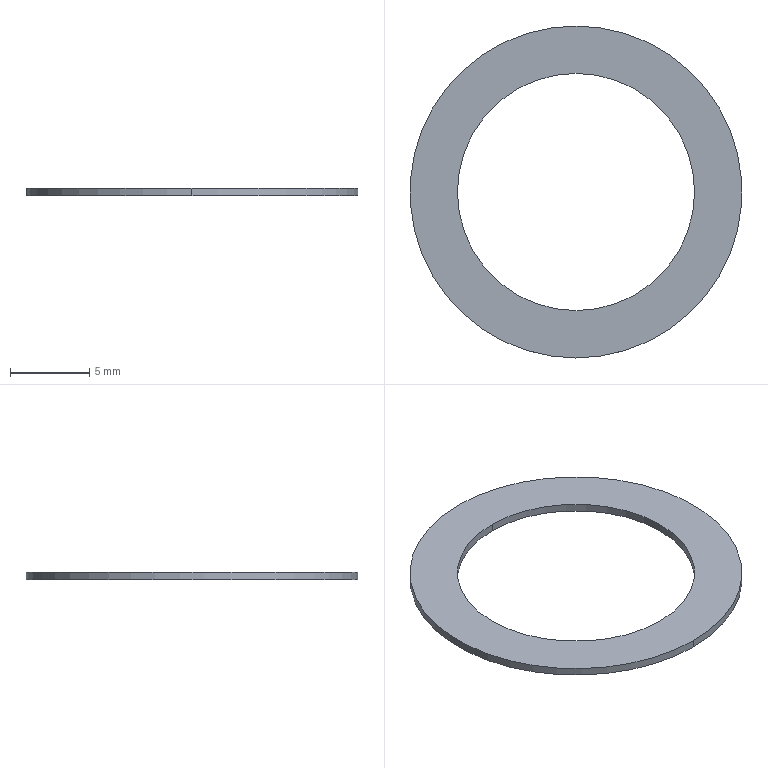Part | STEP file | MSBR-19_1_1_1_1 | 1 solid | 6 faces | box 21 x 21 x 0.5 mm | volume 84.823 mm3 | cylinder 4 | plane 2 | commonest cylinder face diameters 15 x2 21 x2
STEP:
#1=CARTESIAN_POINT('',(0.,0.,0.));
#2=DIRECTION('',(0.,0.,1.));
#3=DIRECTION('',(1.,0.,0.));
#4=AXIS2_PLACEMENT_3D('',#1,#2,#3);
#5=CARTESIAN_POINT('',(-0.000000006,7.5,22.3));
#6=VERTEX_POINT('',#5);
#7=CARTESIAN_POINT('',(-0.000000006,7.5,21.8));
#8=VERTEX_POINT('',#7);
#9=CARTESIAN_POINT('',(-0.000000006,7.5,22.3));
#10=DIRECTION('',(0.,0.,-1.));
#11=VECTOR('',#10,0.5);
#12=LINE('',#9,#11);
#13=EDGE_CURVE('',#6,#8,#12,.T.);
#14=ORIENTED_EDGE('',*,*,#13,.F.);
#15=CARTESIAN_POINT('',(-0.000000006,-7.5,22.3));
#16=VERTEX_POINT('',#15);
#17=CARTESIAN_POINT('',(-0.000000006,-0.000000021,22.3));
#18=DIRECTION('',(0.,0.,1.));
#19=DIRECTION('',(0.,-1.,0.));
#20=AXIS2_PLACEMENT_3D('',#17,#18,#19);
#21=CIRCLE('',#20,7.5);
#22=EDGE_CURVE('',#16,#6,#21,.T.);
#23=ORIENTED_EDGE('',*,*,#22,.F.);
#24=CARTESIAN_POINT('',(-0.000000006,-7.5,21.8));
#25=VERTEX_POINT('',#24);
#26=CARTESIAN_POINT('',(-0.000000006,-7.5,21.8));
#27=DIRECTION('',(0.,0.,1.));
#28=VECTOR('',#27,0.5);
#29=LINE('',#26,#28);
#30=EDGE_CURVE('',#25,#16,#29,.T.);
#31=ORIENTED_EDGE('',*,*,#30,.F.);
#32=CARTESIAN_POINT('',(-0.000000006,-0.000000021,21.8));
#33=DIRECTION('',(0.,0.,-1.));
#34=DIRECTION('',(0.,1.,0.));
#35=AXIS2_PLACEMENT_3D('',#32,#33,#34);
#36=CIRCLE('',#35,7.5);
#37=EDGE_CURVE('',#8,#25,#36,.T.);
#38=ORIENTED_EDGE('',*,*,#37,.F.);
#39=EDGE_LOOP('',(#14,#23,#31,#38));
#40=FACE_OUTER_BOUND('',#39,.F.);
#41=CARTESIAN_POINT('',(-0.000000006,-0.000000021,21.764));
#42=DIRECTION('',(0.,0.,1.));
#43=DIRECTION('',(0.,-1.,0.));
#44=AXIS2_PLACEMENT_3D('',#41,#42,#43);
#45=CYLINDRICAL_SURFACE('',#44,7.5);
#46=ADVANCED_FACE('',(#40),#45,.F.);
#47=CARTESIAN_POINT('',(-0.000000006,-0.000000021,22.3));
#48=DIRECTION('',(0.,0.,1.));
#49=DIRECTION('',(0.,1.,0.));
#50=AXIS2_PLACEMENT_3D('',#47,#48,#49);
#51=CIRCLE('',#50,7.5);
#52=EDGE_CURVE('',#6,#16,#51,.T.);
#53=ORIENTED_EDGE('',*,*,#52,.F.);
#54=ORIENTED_EDGE('',*,*,#13,.T.);
#55=CARTESIAN_POINT('',(-0.000000006,-0.000000021,21.8));
#56=DIRECTION('',(0.,0.,-1.));
#57=DIRECTION('',(0.,-1.,0.));
#58=AXIS2_PLACEMENT_3D('',#55,#56,#57);
#59=CIRCLE('',#58,7.5);
#60=EDGE_CURVE('',#25,#8,#59,.T.);
#61=ORIENTED_EDGE('',*,*,#60,.F.);
#62=ORIENTED_EDGE('',*,*,#30,.T.);
#63=EDGE_LOOP('',(#53,#54,#61,#62));
#64=FACE_OUTER_BOUND('',#63,.F.);
#65=CARTESIAN_POINT('',(-0.000000006,-0.000000021,21.764));
#66=DIRECTION('',(0.,0.,1.));
#67=DIRECTION('',(0.,1.,0.));
#68=AXIS2_PLACEMENT_3D('',#65,#66,#67);
#69=CYLINDRICAL_SURFACE('',#68,7.5);
#70=ADVANCED_FACE('',(#64),#69,.F.);
#71=CARTESIAN_POINT('',(-0.000000006,-10.5,22.3));
#72=VERTEX_POINT('',#71);
#73=CARTESIAN_POINT('',(-0.000000006,10.5,22.3));
#74=VERTEX_POINT('',#73);
#75=CARTESIAN_POINT('',(-0.000000006,-0.000000021,22.3));
#76=DIRECTION('',(0.,0.,-1.));
#77=DIRECTION('',(0.,-1.,0.));
#78=AXIS2_PLACEMENT_3D('',#75,#76,#77);
#79=CIRCLE('',#78,10.5);
#80=EDGE_CURVE('',#72,#74,#79,.T.);
#81=ORIENTED_EDGE('',*,*,#80,.T.);
#82=CARTESIAN_POINT('',(-0.000000006,-0.000000021,22.3));
#83=DIRECTION('',(0.,0.,-1.));
#84=DIRECTION('',(0.,1.,0.));
#85=AXIS2_PLACEMENT_3D('',#82,#83,#84);
#86=CIRCLE('',#85,10.5);
#87=EDGE_CURVE('',#74,#72,#86,.T.);
#88=ORIENTED_EDGE('',*,*,#87,.T.);
#89=EDGE_LOOP('',(#81,#88));
#90=FACE_OUTER_BOUND('',#89,.F.);
#91=ORIENTED_EDGE('',*,*,#22,.T.);
#92=ORIENTED_EDGE('',*,*,#52,.T.);
#93=EDGE_LOOP('',(#91,#92));
#94=FACE_BOUND('',#93,.F.);
#95=CARTESIAN_POINT('',(-0.000000006,-0.000000021,22.3));
#96=DIRECTION('',(0.,0.,1.));
#97=DIRECTION('',(0.,-1.,0.));
#98=AXIS2_PLACEMENT_3D('',#95,#96,#97);
#99=PLANE('',#98);
#100=ADVANCED_FACE('',(#90,#94),#99,.T.);
#101=CARTESIAN_POINT('',(-0.000000006,10.5,21.8));
#102=VERTEX_POINT('',#101);
#103=CARTESIAN_POINT('',(-0.000000006,-10.5,21.8));
#104=VERTEX_POINT('',#103);
#105=CARTESIAN_POINT('',(-0.000000006,-0.000000021,21.8));
#106=DIRECTION('',(0.,0.,1.));
#107=DIRECTION('',(0.,1.,0.));
#108=AXIS2_PLACEMENT_3D('',#105,#106,#107);
#109=CIRCLE('',#108,10.5);
#110=EDGE_CURVE('',#102,#104,#109,.T.);
#111=ORIENTED_EDGE('',*,*,#110,.F.);
#112=CARTESIAN_POINT('',(-0.000000006,10.5,22.3));
#113=DIRECTION('',(0.,0.,-1.));
#114=VECTOR('',#113,0.5);
#115=LINE('',#112,#114);
#116=EDGE_CURVE('',#74,#102,#115,.T.);
#117=ORIENTED_EDGE('',*,*,#116,.F.);
#118=ORIENTED_EDGE('',*,*,#80,.F.);
#119=CARTESIAN_POINT('',(-0.000000006,-10.5,21.8));
#120=DIRECTION('',(0.,0.,1.));
#121=VECTOR('',#120,0.5);
#122=LINE('',#119,#121);
#123=EDGE_CURVE('',#104,#72,#122,.T.);
#124=ORIENTED_EDGE('',*,*,#123,.F.);
#125=EDGE_LOOP('',(#111,#117,#118,#124));
#126=FACE_OUTER_BOUND('',#125,.F.);
#127=CARTESIAN_POINT('',(-0.000000006,-0.000000021,21.764));
#128=DIRECTION('',(0.,0.,1.));
#129=DIRECTION('',(0.,1.,0.));
#130=AXIS2_PLACEMENT_3D('',#127,#128,#129);
#131=CYLINDRICAL_SURFACE('',#130,10.5);
#132=ADVANCED_FACE('',(#126),#131,.T.);
#133=CARTESIAN_POINT('',(-0.000000006,-0.000000021,21.8));
#134=DIRECTION('',(0.,0.,1.));
#135=DIRECTION('',(0.,-1.,0.));
#136=AXIS2_PLACEMENT_3D('',#133,#134,#135);
#137=CIRCLE('',#136,10.5);
#138=EDGE_CURVE('',#104,#102,#137,.T.);
#139=ORIENTED_EDGE('',*,*,#138,.T.);
#140=ORIENTED_EDGE('',*,*,#110,.T.);
#141=EDGE_LOOP('',(#139,#140));
#142=FACE_OUTER_BOUND('',#141,.F.);
#143=ORIENTED_EDGE('',*,*,#37,.T.);
#144=ORIENTED_EDGE('',*,*,#60,.T.);
#145=EDGE_LOOP('',(#143,#144));
#146=FACE_BOUND('',#145,.F.);
#147=CARTESIAN_POINT('',(-0.000000006,-0.000000021,21.8));
#148=DIRECTION('',(0.,0.,1.));
#149=DIRECTION('',(0.,-1.,0.));
#150=AXIS2_PLACEMENT_3D('',#147,#148,#149);
#151=PLANE('',#150);
#152=ADVANCED_FACE('',(#142,#146),#151,.F.);
#153=ORIENTED_EDGE('',*,*,#123,.T.);
#154=ORIENTED_EDGE('',*,*,#87,.F.);
#155=ORIENTED_EDGE('',*,*,#116,.T.);
#156=ORIENTED_EDGE('',*,*,#138,.F.);
#157=EDGE_LOOP('',(#153,#154,#155,#156));
#158=FACE_OUTER_BOUND('',#157,.F.);
#159=CARTESIAN_POINT('',(-0.000000006,-0.000000021,21.764));
#160=DIRECTION('',(0.,0.,1.));
#161=DIRECTION('',(0.,-1.,0.));
#162=AXIS2_PLACEMENT_3D('',#159,#160,#161);
#163=CYLINDRICAL_SURFACE('',#162,10.5);
#164=ADVANCED_FACE('',(#158),#163,.T.);
#165=CLOSED_SHELL('',(#46,#70,#100,#132,#152,#164));
#166=MANIFOLD_SOLID_BREP('',#165);
#167=(LENGTH_UNIT()NAMED_UNIT(*)SI_UNIT(.MILLI.,.METRE.));
#168=UNCERTAINTY_MEASURE_WITH_UNIT(LENGTH_MEASURE(0.002971),#167,'','');
#169=(NAMED_UNIT(*)PLANE_ANGLE_UNIT()SI_UNIT($,.RADIAN.));
#170=PLANE_ANGLE_MEASURE_WITH_UNIT(PLANE_ANGLE_MEASURE(0.01745),#169);
#171=(CONVERSION_BASED_UNIT('DEGREE',#170)NAMED_UNIT(*)PLANE_ANGLE_UNIT());
#172=(NAMED_UNIT(*)SI_UNIT($,.STERADIAN.)SOLID_ANGLE_UNIT());
#173=(GEOMETRIC_REPRESENTATION_CONTEXT(3)GLOBAL_UNCERTAINTY_ASSIGNED_CONTEXT((#168))GLOBAL_UNIT_ASSIGNED_CONTEXT((#167,#171,#172))REPRESENTATION_CONTEXT('',''));
#174=ADVANCED_BREP_SHAPE_REPRESENTATION('',(#4,#166),#173);